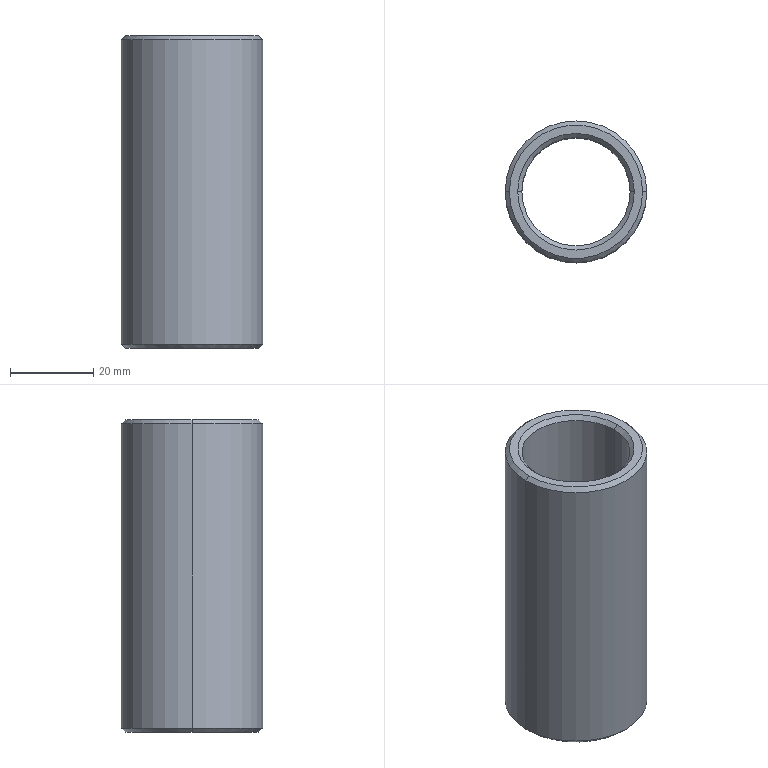Part | SolidWorks | features BaseBody 1 | 1 solid | 14 faces | box 34 x 34 x 75 mm | volume 28086 mm3 | cone 8 | cylinder 4 | plane 2 | commonest cylinder face diameters 26 x2 34 x2
STEP:
#1=CARTESIAN_POINT('',(-16.,0.,-37.5));
#2=VERTEX_POINT('',#1);
#3=CARTESIAN_POINT('',(-17.,0.,-36.5));
#4=VERTEX_POINT('',#3);
#5=CARTESIAN_POINT('',(-17.,0.,-36.5));
#6=DIRECTION('',(-0.7071,0.,0.7071));
#7=VECTOR('',#6,1000.);
#8=LINE('',#5,#7);
#9=EDGE_CURVE('',#2,#4,#8,.T.);
#10=ORIENTED_EDGE('',*,*,#9,.F.);
#11=CARTESIAN_POINT('',(16.,0.,-37.5));
#12=VERTEX_POINT('',#11);
#13=CARTESIAN_POINT('',(0.,0.,-37.5));
#14=DIRECTION('',(0.,0.,-1.));
#15=DIRECTION('',(1.,0.,0.));
#16=AXIS2_PLACEMENT_3D('',#13,#14,#15);
#17=CIRCLE('',#16,16.);
#18=EDGE_CURVE('',#12,#2,#17,.T.);
#19=ORIENTED_EDGE('',*,*,#18,.F.);
#20=CARTESIAN_POINT('',(17.,0.,-36.5));
#21=VERTEX_POINT('',#20);
#22=CARTESIAN_POINT('',(17.,0.,-36.5));
#23=DIRECTION('',(0.7071,0.,0.7071));
#24=VECTOR('',#23,1000.);
#25=LINE('',#22,#24);
#26=EDGE_CURVE('',#12,#21,#25,.T.);
#27=ORIENTED_EDGE('',*,*,#26,.T.);
#28=CARTESIAN_POINT('',(0.,0.,-36.5));
#29=DIRECTION('',(0.,0.,1.));
#30=DIRECTION('',(1.,0.,0.));
#31=AXIS2_PLACEMENT_3D('',#28,#29,#30);
#32=CIRCLE('',#31,17.);
#33=EDGE_CURVE('',#4,#21,#32,.T.);
#34=ORIENTED_EDGE('',*,*,#33,.F.);
#35=EDGE_LOOP('',(#10,#19,#27,#34));
#36=FACE_OUTER_BOUND('',#35,.T.);
#37=CARTESIAN_POINT('',(0.,0.,-36.5));
#38=DIRECTION('',(0.,0.,1.));
#39=DIRECTION('',(1.,0.,0.));
#40=AXIS2_PLACEMENT_3D('',#37,#38,#39);
#41=CONICAL_SURFACE('',#40,17.,0.7854);
#42=ADVANCED_FACE('',(#36),#41,.T.);
#43=CARTESIAN_POINT('',(-13.,0.,36.5));
#44=VERTEX_POINT('',#43);
#45=CARTESIAN_POINT('',(-14.,0.,37.5));
#46=VERTEX_POINT('',#45);
#47=CARTESIAN_POINT('',(-13.,0.,36.5));
#48=DIRECTION('',(-0.7071,0.,0.7071));
#49=VECTOR('',#48,1000.);
#50=LINE('',#47,#49);
#51=EDGE_CURVE('',#44,#46,#50,.T.);
#52=ORIENTED_EDGE('',*,*,#51,.F.);
#53=CARTESIAN_POINT('',(13.,0.,36.5));
#54=VERTEX_POINT('',#53);
#55=CARTESIAN_POINT('',(0.,0.,36.5));
#56=DIRECTION('',(0.,0.,1.));
#57=DIRECTION('',(1.,0.,0.));
#58=AXIS2_PLACEMENT_3D('',#55,#56,#57);
#59=CIRCLE('',#58,13.);
#60=EDGE_CURVE('',#54,#44,#59,.T.);
#61=ORIENTED_EDGE('',*,*,#60,.F.);
#62=CARTESIAN_POINT('',(14.,0.,37.5));
#63=VERTEX_POINT('',#62);
#64=CARTESIAN_POINT('',(13.,0.,36.5));
#65=DIRECTION('',(0.7071,0.,0.7071));
#66=VECTOR('',#65,1000.);
#67=LINE('',#64,#66);
#68=EDGE_CURVE('',#54,#63,#67,.T.);
#69=ORIENTED_EDGE('',*,*,#68,.T.);
#70=CARTESIAN_POINT('',(0.,0.,37.5));
#71=DIRECTION('',(0.,0.,-1.));
#72=DIRECTION('',(1.,0.,0.));
#73=AXIS2_PLACEMENT_3D('',#70,#71,#72);
#74=CIRCLE('',#73,14.);
#75=EDGE_CURVE('',#46,#63,#74,.T.);
#76=ORIENTED_EDGE('',*,*,#75,.F.);
#77=EDGE_LOOP('',(#52,#61,#69,#76));
#78=FACE_OUTER_BOUND('',#77,.T.);
#79=CARTESIAN_POINT('',(0.,0.,36.5));
#80=DIRECTION('',(0.,0.,1.));
#81=DIRECTION('',(1.,0.,0.));
#82=AXIS2_PLACEMENT_3D('',#79,#80,#81);
#83=CONICAL_SURFACE('',#82,13.,0.7854);
#84=ADVANCED_FACE('',(#78),#83,.F.);
#85=CARTESIAN_POINT('',(16.,0.,37.5));
#86=VERTEX_POINT('',#85);
#87=CARTESIAN_POINT('',(17.,0.,36.5));
#88=VERTEX_POINT('',#87);
#89=CARTESIAN_POINT('',(16.,0.,37.5));
#90=DIRECTION('',(0.7071,0.,-0.7071));
#91=VECTOR('',#90,1000.);
#92=LINE('',#89,#91);
#93=EDGE_CURVE('',#86,#88,#92,.T.);
#94=ORIENTED_EDGE('',*,*,#93,.F.);
#95=CARTESIAN_POINT('',(-16.,0.,37.5));
#96=VERTEX_POINT('',#95);
#97=CARTESIAN_POINT('',(0.,0.,37.5));
#98=DIRECTION('',(0.,0.,1.));
#99=DIRECTION('',(1.,0.,0.));
#100=AXIS2_PLACEMENT_3D('',#97,#98,#99);
#101=CIRCLE('',#100,16.);
#102=EDGE_CURVE('',#96,#86,#101,.T.);
#103=ORIENTED_EDGE('',*,*,#102,.F.);
#104=CARTESIAN_POINT('',(-17.,0.,36.5));
#105=VERTEX_POINT('',#104);
#106=CARTESIAN_POINT('',(-16.,0.,37.5));
#107=DIRECTION('',(-0.7071,0.,-0.7071));
#108=VECTOR('',#107,1000.);
#109=LINE('',#106,#108);
#110=EDGE_CURVE('',#96,#105,#109,.T.);
#111=ORIENTED_EDGE('',*,*,#110,.T.);
#112=CARTESIAN_POINT('',(0.,0.,36.5));
#113=DIRECTION('',(0.,0.,-1.));
#114=DIRECTION('',(1.,0.,0.));
#115=AXIS2_PLACEMENT_3D('',#112,#113,#114);
#116=CIRCLE('',#115,17.);
#117=EDGE_CURVE('',#88,#105,#116,.T.);
#118=ORIENTED_EDGE('',*,*,#117,.F.);
#119=EDGE_LOOP('',(#94,#103,#111,#118));
#120=FACE_OUTER_BOUND('',#119,.T.);
#121=CARTESIAN_POINT('',(0.,0.,37.5));
#122=DIRECTION('',(0.,0.,-1.));
#123=DIRECTION('',(-1.,0.,0.));
#124=AXIS2_PLACEMENT_3D('',#121,#122,#123);
#125=CONICAL_SURFACE('',#124,16.,0.7854);
#126=ADVANCED_FACE('',(#120),#125,.T.);
#127=CARTESIAN_POINT('',(13.,0.,-36.5));
#128=VERTEX_POINT('',#127);
#129=CARTESIAN_POINT('',(14.,0.,-37.5));
#130=VERTEX_POINT('',#129);
#131=CARTESIAN_POINT('',(14.,0.,-37.5));
#132=DIRECTION('',(0.7071,0.,-0.7071));
#133=VECTOR('',#132,1000.);
#134=LINE('',#131,#133);
#135=EDGE_CURVE('',#128,#130,#134,.T.);
#136=ORIENTED_EDGE('',*,*,#135,.F.);
#137=CARTESIAN_POINT('',(-13.,0.,-36.5));
#138=VERTEX_POINT('',#137);
#139=CARTESIAN_POINT('',(0.,0.,-36.5));
#140=DIRECTION('',(0.,0.,-1.));
#141=DIRECTION('',(1.,0.,0.));
#142=AXIS2_PLACEMENT_3D('',#139,#140,#141);
#143=CIRCLE('',#142,13.);
#144=EDGE_CURVE('',#138,#128,#143,.T.);
#145=ORIENTED_EDGE('',*,*,#144,.F.);
#146=CARTESIAN_POINT('',(-14.,0.,-37.5));
#147=VERTEX_POINT('',#146);
#148=CARTESIAN_POINT('',(-14.,0.,-37.5));
#149=DIRECTION('',(-0.7071,0.,-0.7071));
#150=VECTOR('',#149,1000.);
#151=LINE('',#148,#150);
#152=EDGE_CURVE('',#138,#147,#151,.T.);
#153=ORIENTED_EDGE('',*,*,#152,.T.);
#154=CARTESIAN_POINT('',(0.,0.,-37.5));
#155=DIRECTION('',(0.,0.,1.));
#156=DIRECTION('',(1.,0.,0.));
#157=AXIS2_PLACEMENT_3D('',#154,#155,#156);
#158=CIRCLE('',#157,14.);
#159=EDGE_CURVE('',#130,#147,#158,.T.);
#160=ORIENTED_EDGE('',*,*,#159,.F.);
#161=EDGE_LOOP('',(#136,#145,#153,#160));
#162=FACE_OUTER_BOUND('',#161,.T.);
#163=CARTESIAN_POINT('',(0.,0.,-37.5));
#164=DIRECTION('',(0.,0.,-1.));
#165=DIRECTION('',(-1.,0.,0.));
#166=AXIS2_PLACEMENT_3D('',#163,#164,#165);
#167=CONICAL_SURFACE('',#166,14.,0.7854);
#168=ADVANCED_FACE('',(#162),#167,.F.);
#169=CARTESIAN_POINT('',(-13.,0.,-37.5));
#170=DIRECTION('',(0.,0.,1.));
#171=VECTOR('',#170,1000.);
#172=LINE('',#169,#171);
#173=EDGE_CURVE('',#138,#44,#172,.T.);
#174=ORIENTED_EDGE('',*,*,#173,.F.);
#175=ORIENTED_EDGE('',*,*,#144,.T.);
#176=CARTESIAN_POINT('',(13.,0.,-37.5));
#177=DIRECTION('',(0.,0.,1.));
#178=VECTOR('',#177,1000.);
#179=LINE('',#176,#178);
#180=EDGE_CURVE('',#128,#54,#179,.T.);
#181=ORIENTED_EDGE('',*,*,#180,.T.);
#182=ORIENTED_EDGE('',*,*,#60,.T.);
#183=EDGE_LOOP('',(#174,#175,#181,#182));
#184=FACE_OUTER_BOUND('',#183,.T.);
#185=CARTESIAN_POINT('',(0.,0.,-37.5));
#186=DIRECTION('',(0.,0.,1.));
#187=DIRECTION('',(1.,0.,0.));
#188=AXIS2_PLACEMENT_3D('',#185,#186,#187);
#189=CYLINDRICAL_SURFACE('',#188,13.);
#190=ADVANCED_FACE('',(#184),#189,.F.);
#191=CARTESIAN_POINT('',(0.,0.,37.5));
#192=DIRECTION('',(0.,0.,-1.));
#193=DIRECTION('',(1.,0.,0.));
#194=AXIS2_PLACEMENT_3D('',#191,#192,#193);
#195=CIRCLE('',#194,14.);
#196=EDGE_CURVE('',#63,#46,#195,.T.);
#197=ORIENTED_EDGE('',*,*,#196,.T.);
#198=ORIENTED_EDGE('',*,*,#75,.T.);
#199=EDGE_LOOP('',(#197,#198));
#200=FACE_BOUND('',#199,.T.);
#201=ORIENTED_EDGE('',*,*,#102,.T.);
#202=CARTESIAN_POINT('',(0.,0.,37.5));
#203=DIRECTION('',(0.,0.,1.));
#204=DIRECTION('',(1.,0.,0.));
#205=AXIS2_PLACEMENT_3D('',#202,#203,#204);
#206=CIRCLE('',#205,16.);
#207=EDGE_CURVE('',#86,#96,#206,.T.);
#208=ORIENTED_EDGE('',*,*,#207,.T.);
#209=EDGE_LOOP('',(#201,#208));
#210=FACE_OUTER_BOUND('',#209,.T.);
#211=CARTESIAN_POINT('',(0.,0.,37.5));
#212=DIRECTION('',(0.,0.,1.));
#213=DIRECTION('',(1.,0.,0.));
#214=AXIS2_PLACEMENT_3D('',#211,#212,#213);
#215=PLANE('',#214);
#216=ADVANCED_FACE('',(#200,#210),#215,.T.);
#217=CARTESIAN_POINT('',(0.,0.,-37.5));
#218=DIRECTION('',(0.,0.,1.));
#219=DIRECTION('',(1.,0.,0.));
#220=AXIS2_PLACEMENT_3D('',#217,#218,#219);
#221=CIRCLE('',#220,14.);
#222=EDGE_CURVE('',#147,#130,#221,.T.);
#223=ORIENTED_EDGE('',*,*,#222,.T.);
#224=ORIENTED_EDGE('',*,*,#159,.T.);
#225=EDGE_LOOP('',(#223,#224));
#226=FACE_BOUND('',#225,.T.);
#227=ORIENTED_EDGE('',*,*,#18,.T.);
#228=CARTESIAN_POINT('',(0.,0.,-37.5));
#229=DIRECTION('',(0.,0.,-1.));
#230=DIRECTION('',(1.,0.,0.));
#231=AXIS2_PLACEMENT_3D('',#228,#229,#230);
#232=CIRCLE('',#231,16.);
#233=EDGE_CURVE('',#2,#12,#232,.T.);
#234=ORIENTED_EDGE('',*,*,#233,.T.);
#235=EDGE_LOOP('',(#227,#234));
#236=FACE_OUTER_BOUND('',#235,.T.);
#237=CARTESIAN_POINT('',(0.,0.,-37.5));
#238=DIRECTION('',(0.,0.,1.));
#239=DIRECTION('',(1.,0.,0.));
#240=AXIS2_PLACEMENT_3D('',#237,#238,#239);
#241=PLANE('',#240);
#242=ADVANCED_FACE('',(#226,#236),#241,.F.);
#243=CARTESIAN_POINT('',(-17.,0.,-37.5));
#244=DIRECTION('',(0.,0.,1.));
#245=VECTOR('',#244,1000.);
#246=LINE('',#243,#245);
#247=EDGE_CURVE('',#4,#105,#246,.T.);
#248=ORIENTED_EDGE('',*,*,#247,.F.);
#249=ORIENTED_EDGE('',*,*,#33,.T.);
#250=CARTESIAN_POINT('',(17.,0.,-37.5));
#251=DIRECTION('',(0.,0.,1.));
#252=VECTOR('',#251,1000.);
#253=LINE('',#250,#252);
#254=EDGE_CURVE('',#21,#88,#253,.T.);
#255=ORIENTED_EDGE('',*,*,#254,.T.);
#256=ORIENTED_EDGE('',*,*,#117,.T.);
#257=EDGE_LOOP('',(#248,#249,#255,#256));
#258=FACE_OUTER_BOUND('',#257,.T.);
#259=CARTESIAN_POINT('',(0.,0.,-37.5));
#260=DIRECTION('',(0.,0.,1.));
#261=DIRECTION('',(1.,0.,0.));
#262=AXIS2_PLACEMENT_3D('',#259,#260,#261);
#263=CYLINDRICAL_SURFACE('',#262,17.);
#264=ADVANCED_FACE('',(#258),#263,.T.);
#265=CARTESIAN_POINT('',(0.,0.,-36.5));
#266=DIRECTION('',(0.,0.,1.));
#267=DIRECTION('',(1.,0.,0.));
#268=AXIS2_PLACEMENT_3D('',#265,#266,#267);
#269=CIRCLE('',#268,17.);
#270=EDGE_CURVE('',#21,#4,#269,.T.);
#271=ORIENTED_EDGE('',*,*,#270,.T.);
#272=ORIENTED_EDGE('',*,*,#247,.T.);
#273=CARTESIAN_POINT('',(0.,0.,36.5));
#274=DIRECTION('',(0.,0.,-1.));
#275=DIRECTION('',(1.,0.,0.));
#276=AXIS2_PLACEMENT_3D('',#273,#274,#275);
#277=CIRCLE('',#276,17.);
#278=EDGE_CURVE('',#105,#88,#277,.T.);
#279=ORIENTED_EDGE('',*,*,#278,.T.);
#280=ORIENTED_EDGE('',*,*,#254,.F.);
#281=EDGE_LOOP('',(#271,#272,#279,#280));
#282=FACE_OUTER_BOUND('',#281,.T.);
#283=CARTESIAN_POINT('',(0.,0.,-37.5));
#284=DIRECTION('',(0.,0.,1.));
#285=DIRECTION('',(1.,0.,0.));
#286=AXIS2_PLACEMENT_3D('',#283,#284,#285);
#287=CYLINDRICAL_SURFACE('',#286,17.);
#288=ADVANCED_FACE('',(#282),#287,.T.);
#289=CARTESIAN_POINT('',(0.,0.,-36.5));
#290=DIRECTION('',(0.,0.,-1.));
#291=DIRECTION('',(1.,0.,0.));
#292=AXIS2_PLACEMENT_3D('',#289,#290,#291);
#293=CIRCLE('',#292,13.);
#294=EDGE_CURVE('',#128,#138,#293,.T.);
#295=ORIENTED_EDGE('',*,*,#294,.T.);
#296=ORIENTED_EDGE('',*,*,#173,.T.);
#297=CARTESIAN_POINT('',(0.,0.,36.5));
#298=DIRECTION('',(0.,0.,1.));
#299=DIRECTION('',(1.,0.,0.));
#300=AXIS2_PLACEMENT_3D('',#297,#298,#299);
#301=CIRCLE('',#300,13.);
#302=EDGE_CURVE('',#44,#54,#301,.T.);
#303=ORIENTED_EDGE('',*,*,#302,.T.);
#304=ORIENTED_EDGE('',*,*,#180,.F.);
#305=EDGE_LOOP('',(#295,#296,#303,#304));
#306=FACE_OUTER_BOUND('',#305,.T.);
#307=CARTESIAN_POINT('',(0.,0.,-37.5));
#308=DIRECTION('',(0.,0.,1.));
#309=DIRECTION('',(1.,0.,0.));
#310=AXIS2_PLACEMENT_3D('',#307,#308,#309);
#311=CYLINDRICAL_SURFACE('',#310,13.);
#312=ADVANCED_FACE('',(#306),#311,.F.);
#313=ORIENTED_EDGE('',*,*,#294,.F.);
#314=ORIENTED_EDGE('',*,*,#135,.T.);
#315=ORIENTED_EDGE('',*,*,#222,.F.);
#316=ORIENTED_EDGE('',*,*,#152,.F.);
#317=EDGE_LOOP('',(#313,#314,#315,#316));
#318=FACE_OUTER_BOUND('',#317,.T.);
#319=CARTESIAN_POINT('',(0.,0.,-37.5));
#320=DIRECTION('',(0.,0.,-1.));
#321=DIRECTION('',(-1.,0.,0.));
#322=AXIS2_PLACEMENT_3D('',#319,#320,#321);
#323=CONICAL_SURFACE('',#322,14.,0.7854);
#324=ADVANCED_FACE('',(#318),#323,.F.);
#325=ORIENTED_EDGE('',*,*,#207,.F.);
#326=ORIENTED_EDGE('',*,*,#93,.T.);
#327=ORIENTED_EDGE('',*,*,#278,.F.);
#328=ORIENTED_EDGE('',*,*,#110,.F.);
#329=EDGE_LOOP('',(#325,#326,#327,#328));
#330=FACE_OUTER_BOUND('',#329,.T.);
#331=CARTESIAN_POINT('',(0.,0.,37.5));
#332=DIRECTION('',(0.,0.,-1.));
#333=DIRECTION('',(-1.,0.,0.));
#334=AXIS2_PLACEMENT_3D('',#331,#332,#333);
#335=CONICAL_SURFACE('',#334,16.,0.7854);
#336=ADVANCED_FACE('',(#330),#335,.T.);
#337=ORIENTED_EDGE('',*,*,#302,.F.);
#338=ORIENTED_EDGE('',*,*,#51,.T.);
#339=ORIENTED_EDGE('',*,*,#196,.F.);
#340=ORIENTED_EDGE('',*,*,#68,.F.);
#341=EDGE_LOOP('',(#337,#338,#339,#340));
#342=FACE_OUTER_BOUND('',#341,.T.);
#343=CARTESIAN_POINT('',(0.,0.,36.5));
#344=DIRECTION('',(0.,0.,1.));
#345=DIRECTION('',(1.,0.,0.));
#346=AXIS2_PLACEMENT_3D('',#343,#344,#345);
#347=CONICAL_SURFACE('',#346,13.,0.7854);
#348=ADVANCED_FACE('',(#342),#347,.F.);
#349=ORIENTED_EDGE('',*,*,#233,.F.);
#350=ORIENTED_EDGE('',*,*,#9,.T.);
#351=ORIENTED_EDGE('',*,*,#270,.F.);
#352=ORIENTED_EDGE('',*,*,#26,.F.);
#353=EDGE_LOOP('',(#349,#350,#351,#352));
#354=FACE_OUTER_BOUND('',#353,.T.);
#355=CARTESIAN_POINT('',(0.,0.,-36.5));
#356=DIRECTION('',(0.,0.,1.));
#357=DIRECTION('',(1.,0.,0.));
#358=AXIS2_PLACEMENT_3D('',#355,#356,#357);
#359=CONICAL_SURFACE('',#358,17.,0.7854);
#360=ADVANCED_FACE('',(#354),#359,.T.);
#361=CLOSED_SHELL('',(#42,#84,#126,#168,#190,#216,#242,#264,#288,#312,#324,#336,#348,#360));
#362=MANIFOLD_SOLID_BREP('',#361);
#363=CARTESIAN_POINT('',(0.,0.,0.));
#364=DIRECTION('',(0.,0.,1.));
#365=DIRECTION('',(1.,0.,0.));
#366=AXIS2_PLACEMENT_3D('',#363,#364,#365);
#367=(LENGTH_UNIT()NAMED_UNIT(*)SI_UNIT(.MILLI.,.METRE.));
#368=UNCERTAINTY_MEASURE_WITH_UNIT(LENGTH_MEASURE(0.00001),#367,'','');
#369=(NAMED_UNIT(*)PLANE_ANGLE_UNIT()SI_UNIT($,.RADIAN.));
#370=(NAMED_UNIT(*)SI_UNIT($,.STERADIAN.)SOLID_ANGLE_UNIT());
#371=(GEOMETRIC_REPRESENTATION_CONTEXT(3)GLOBAL_UNCERTAINTY_ASSIGNED_CONTEXT((#368))GLOBAL_UNIT_ASSIGNED_CONTEXT((#367,#369,#370))REPRESENTATION_CONTEXT('',''));
#372=ADVANCED_BREP_SHAPE_REPRESENTATION('',(#362,#366),#371);